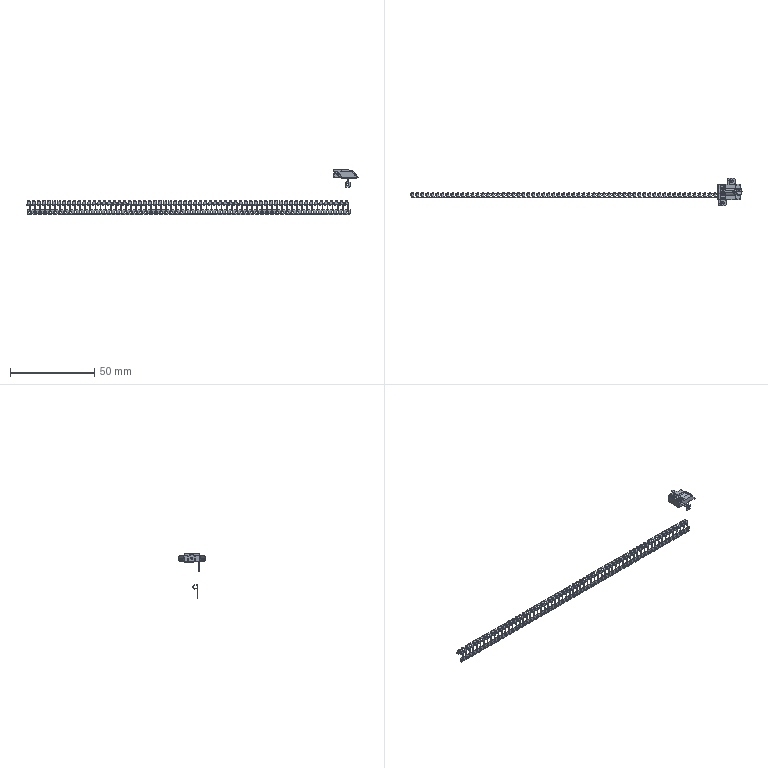Part | NX | 5 solids | 8131 faces | volume 547.656 mm3 | plane 3572 | cylinder 2857 | torus 1354 | sphere 308 | spline 22 | cone 18 | commonest cylinder face diameters 0.2 x628 0.8 x331 0.4 x280 0.6 x266 0.12 x260 0.44 x260